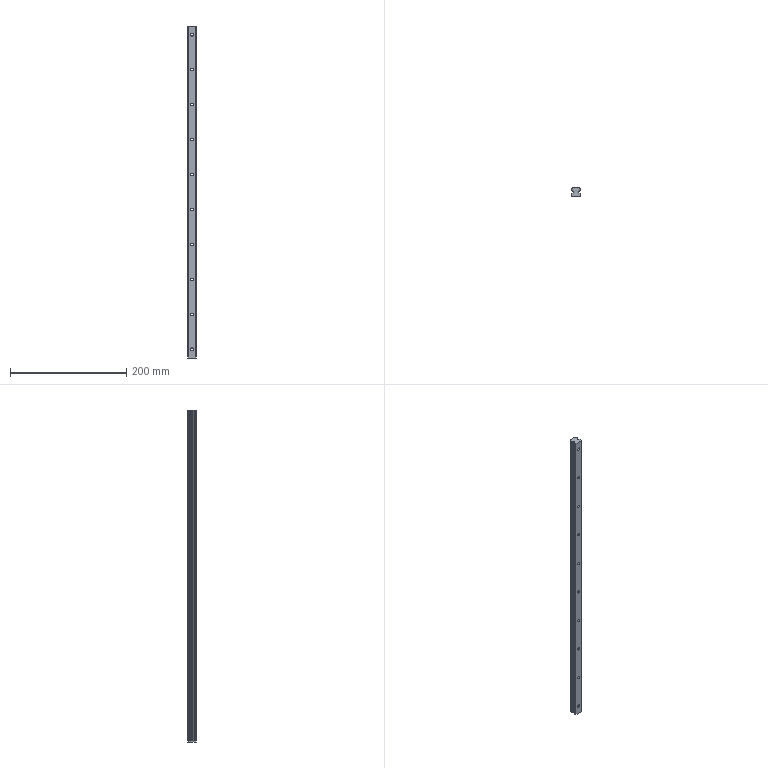Part | STEP file | HGR15-570 | 1 solid | 86 faces | box 15 x 15 x 570 mm | volume 104849 mm3 | cylinder 54 | plane 32 | commonest cylinder face diameters 4.5 x20 7.5 x20 0.8 x8 3.24 x4 2 x2